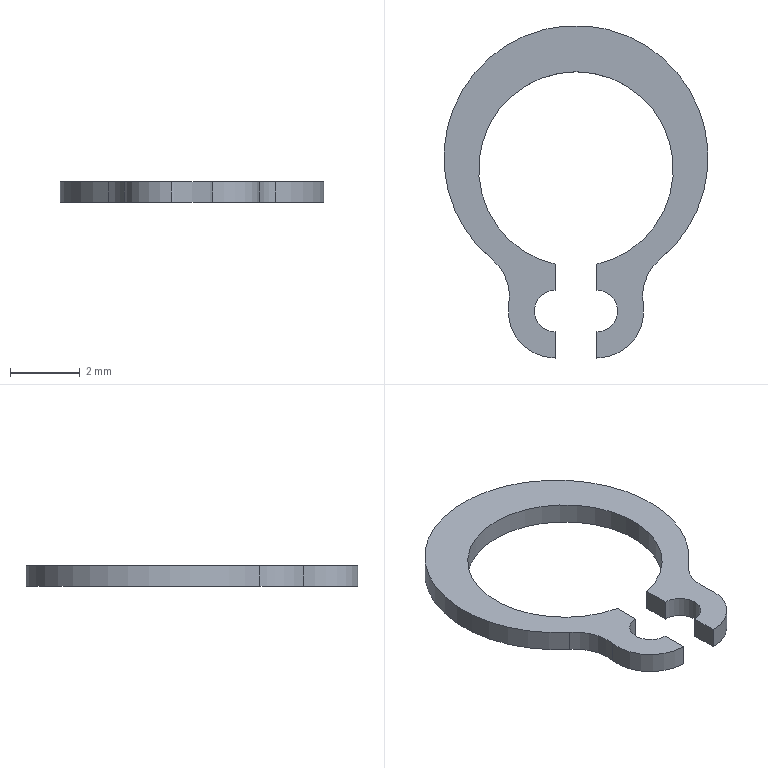Part | NX | features BREP 1, DATUM_CSYS 1 | 1 solid | 14 faces | box 7.6 x 9.565 x 0.6 mm | volume 14.427 mm3 | cylinder 8 | plane 6 | commonest cylinder face diameters 2.7 x4 1.2 x2 5.6 x1 7.6 x1
STEP:
#1=CARTESIAN_POINT('',(-0.6,-2.735,0.));
#2=VERTEX_POINT('',#1);
#3=CARTESIAN_POINT('',(0.6,-2.735,0.));
#4=VERTEX_POINT('',#3);
#5=CARTESIAN_POINT('',(0.,0.,0.));
#6=DIRECTION('',(0.,0.,-1.));
#7=DIRECTION('',(-0.2143,-0.9768,0.));
#8=AXIS2_PLACEMENT_3D('',#5,#6,#7);
#9=CIRCLE('',#8,2.8);
#10=EDGE_CURVE('',#2,#4,#9,.T.);
#11=ORIENTED_EDGE('',*,*,#10,.F.);
#12=CARTESIAN_POINT('',(-0.6,-3.485,0.));
#13=VERTEX_POINT('',#12);
#14=CARTESIAN_POINT('',(-0.6,-3.485,0.));
#15=DIRECTION('',(0.,1.,0.));
#16=VECTOR('',#15,1000.);
#17=LINE('',#14,#16);
#18=EDGE_CURVE('',#13,#2,#17,.T.);
#19=ORIENTED_EDGE('',*,*,#18,.F.);
#20=CARTESIAN_POINT('',(-0.6,-4.685,0.));
#21=VERTEX_POINT('',#20);
#22=CARTESIAN_POINT('',(-0.6,-4.085,0.));
#23=DIRECTION('',(0.,0.,-1.));
#24=DIRECTION('',(0.,-1.,0.));
#25=AXIS2_PLACEMENT_3D('',#22,#23,#24);
#26=CIRCLE('',#25,0.6);
#27=EDGE_CURVE('',#21,#13,#26,.T.);
#28=ORIENTED_EDGE('',*,*,#27,.F.);
#29=CARTESIAN_POINT('',(-0.6,-5.435,0.));
#30=VERTEX_POINT('',#29);
#31=CARTESIAN_POINT('',(-0.6,-5.435,0.));
#32=DIRECTION('',(0.,1.,0.));
#33=VECTOR('',#32,1000.);
#34=LINE('',#31,#33);
#35=EDGE_CURVE('',#30,#21,#34,.T.);
#36=ORIENTED_EDGE('',*,*,#35,.F.);
#37=CARTESIAN_POINT('',(-1.933,-3.869,0.));
#38=VERTEX_POINT('',#37);
#39=CARTESIAN_POINT('',(-0.6,-4.085,0.));
#40=DIRECTION('',(0.,0.,1.));
#41=DIRECTION('',(-0.9871,0.1601,0.));
#42=AXIS2_PLACEMENT_3D('',#39,#40,#41);
#43=CIRCLE('',#42,1.35);
#44=EDGE_CURVE('',#38,#30,#43,.T.);
#45=ORIENTED_EDGE('',*,*,#44,.F.);
#46=CARTESIAN_POINT('',(-2.409,-2.609,0.));
#47=VERTEX_POINT('',#46);
#48=CARTESIAN_POINT('',(-3.265,-3.653,0.));
#49=DIRECTION('',(0.,0.,-1.));
#50=DIRECTION('',(0.634,0.7733,0.));
#51=AXIS2_PLACEMENT_3D('',#48,#49,#50);
#52=CIRCLE('',#51,1.35);
#53=EDGE_CURVE('',#47,#38,#52,.T.);
#54=ORIENTED_EDGE('',*,*,#53,.F.);
#55=CARTESIAN_POINT('',(2.409,-2.609,0.));
#56=VERTEX_POINT('',#55);
#57=CARTESIAN_POINT('',(0.,0.33,0.));
#58=DIRECTION('',(0.,0.,1.));
#59=DIRECTION('',(0.634,-0.7733,0.));
#60=AXIS2_PLACEMENT_3D('',#57,#58,#59);
#61=CIRCLE('',#60,3.8);
#62=EDGE_CURVE('',#56,#47,#61,.T.);
#63=ORIENTED_EDGE('',*,*,#62,.F.);
#64=CARTESIAN_POINT('',(1.933,-3.869,0.));
#65=VERTEX_POINT('',#64);
#66=CARTESIAN_POINT('',(3.265,-3.653,0.));
#67=DIRECTION('',(0.,0.,-1.));
#68=DIRECTION('',(-0.9871,-0.1601,0.));
#69=AXIS2_PLACEMENT_3D('',#66,#67,#68);
#70=CIRCLE('',#69,1.35);
#71=EDGE_CURVE('',#65,#56,#70,.T.);
#72=ORIENTED_EDGE('',*,*,#71,.F.);
#73=CARTESIAN_POINT('',(0.6,-5.435,0.));
#74=VERTEX_POINT('',#73);
#75=CARTESIAN_POINT('',(0.6,-4.085,0.));
#76=DIRECTION('',(0.,0.,1.));
#77=DIRECTION('',(0.,-1.,0.));
#78=AXIS2_PLACEMENT_3D('',#75,#76,#77);
#79=CIRCLE('',#78,1.35);
#80=EDGE_CURVE('',#74,#65,#79,.T.);
#81=ORIENTED_EDGE('',*,*,#80,.F.);
#82=CARTESIAN_POINT('',(0.6,-4.685,0.));
#83=VERTEX_POINT('',#82);
#84=CARTESIAN_POINT('',(0.6,-4.685,0.));
#85=DIRECTION('',(0.,-1.,0.));
#86=VECTOR('',#85,1000.);
#87=LINE('',#84,#86);
#88=EDGE_CURVE('',#83,#74,#87,.T.);
#89=ORIENTED_EDGE('',*,*,#88,.F.);
#90=CARTESIAN_POINT('',(0.6,-3.485,0.));
#91=VERTEX_POINT('',#90);
#92=CARTESIAN_POINT('',(0.6,-4.085,0.));
#93=DIRECTION('',(0.,0.,-1.));
#94=DIRECTION('',(0.,1.,0.));
#95=AXIS2_PLACEMENT_3D('',#92,#93,#94);
#96=CIRCLE('',#95,0.6);
#97=EDGE_CURVE('',#91,#83,#96,.T.);
#98=ORIENTED_EDGE('',*,*,#97,.F.);
#99=CARTESIAN_POINT('',(0.6,-2.735,0.));
#100=DIRECTION('',(0.,-1.,0.));
#101=VECTOR('',#100,1000.);
#102=LINE('',#99,#101);
#103=EDGE_CURVE('',#4,#91,#102,.T.);
#104=ORIENTED_EDGE('',*,*,#103,.F.);
#105=EDGE_LOOP('',(#11,#19,#28,#36,#45,#54,#63,#72,#81,#89,#98,#104));
#106=FACE_BOUND('',#105,.T.);
#107=CARTESIAN_POINT('',(0.3031,-0.6525,0.));
#108=DIRECTION('',(0.,0.,1.));
#109=DIRECTION('',(-1.,0.,0.));
#110=AXIS2_PLACEMENT_3D('',#107,#108,#109);
#111=PLANE('',#110);
#112=ADVANCED_FACE('',(#106),#111,.F.);
#113=CARTESIAN_POINT('',(0.6,-2.735,0.6));
#114=VERTEX_POINT('',#113);
#115=CARTESIAN_POINT('',(0.6,-3.485,0.6));
#116=VERTEX_POINT('',#115);
#117=CARTESIAN_POINT('',(0.6,-2.735,0.6));
#118=DIRECTION('',(0.,-1.,0.));
#119=VECTOR('',#118,1000.);
#120=LINE('',#117,#119);
#121=EDGE_CURVE('',#114,#116,#120,.T.);
#122=ORIENTED_EDGE('',*,*,#121,.T.);
#123=CARTESIAN_POINT('',(0.6,-4.685,0.6));
#124=VERTEX_POINT('',#123);
#125=CARTESIAN_POINT('',(0.6,-4.085,0.6));
#126=DIRECTION('',(0.,0.,-1.));
#127=DIRECTION('',(0.,1.,0.));
#128=AXIS2_PLACEMENT_3D('',#125,#126,#127);
#129=CIRCLE('',#128,0.6);
#130=EDGE_CURVE('',#116,#124,#129,.T.);
#131=ORIENTED_EDGE('',*,*,#130,.T.);
#132=CARTESIAN_POINT('',(0.6,-5.435,0.6));
#133=VERTEX_POINT('',#132);
#134=CARTESIAN_POINT('',(0.6,-4.685,0.6));
#135=DIRECTION('',(0.,-1.,0.));
#136=VECTOR('',#135,1000.);
#137=LINE('',#134,#136);
#138=EDGE_CURVE('',#124,#133,#137,.T.);
#139=ORIENTED_EDGE('',*,*,#138,.T.);
#140=CARTESIAN_POINT('',(1.933,-3.869,0.6));
#141=VERTEX_POINT('',#140);
#142=CARTESIAN_POINT('',(0.6,-4.085,0.6));
#143=DIRECTION('',(0.,0.,1.));
#144=DIRECTION('',(0.,-1.,0.));
#145=AXIS2_PLACEMENT_3D('',#142,#143,#144);
#146=CIRCLE('',#145,1.35);
#147=EDGE_CURVE('',#133,#141,#146,.T.);
#148=ORIENTED_EDGE('',*,*,#147,.T.);
#149=CARTESIAN_POINT('',(2.409,-2.609,0.6));
#150=VERTEX_POINT('',#149);
#151=CARTESIAN_POINT('',(3.265,-3.653,0.6));
#152=DIRECTION('',(0.,0.,-1.));
#153=DIRECTION('',(-0.9871,-0.1601,0.));
#154=AXIS2_PLACEMENT_3D('',#151,#152,#153);
#155=CIRCLE('',#154,1.35);
#156=EDGE_CURVE('',#141,#150,#155,.T.);
#157=ORIENTED_EDGE('',*,*,#156,.T.);
#158=CARTESIAN_POINT('',(-2.409,-2.609,0.6));
#159=VERTEX_POINT('',#158);
#160=CARTESIAN_POINT('',(0.,0.33,0.6));
#161=DIRECTION('',(0.,0.,1.));
#162=DIRECTION('',(0.634,-0.7733,0.));
#163=AXIS2_PLACEMENT_3D('',#160,#161,#162);
#164=CIRCLE('',#163,3.8);
#165=EDGE_CURVE('',#150,#159,#164,.T.);
#166=ORIENTED_EDGE('',*,*,#165,.T.);
#167=CARTESIAN_POINT('',(-1.933,-3.869,0.6));
#168=VERTEX_POINT('',#167);
#169=CARTESIAN_POINT('',(-3.265,-3.653,0.6));
#170=DIRECTION('',(0.,0.,-1.));
#171=DIRECTION('',(0.634,0.7733,0.));
#172=AXIS2_PLACEMENT_3D('',#169,#170,#171);
#173=CIRCLE('',#172,1.35);
#174=EDGE_CURVE('',#159,#168,#173,.T.);
#175=ORIENTED_EDGE('',*,*,#174,.T.);
#176=CARTESIAN_POINT('',(-0.6,-5.435,0.6));
#177=VERTEX_POINT('',#176);
#178=CARTESIAN_POINT('',(-0.6,-4.085,0.6));
#179=DIRECTION('',(0.,0.,1.));
#180=DIRECTION('',(-0.9871,0.1601,0.));
#181=AXIS2_PLACEMENT_3D('',#178,#179,#180);
#182=CIRCLE('',#181,1.35);
#183=EDGE_CURVE('',#168,#177,#182,.T.);
#184=ORIENTED_EDGE('',*,*,#183,.T.);
#185=CARTESIAN_POINT('',(-0.6,-4.685,0.6));
#186=VERTEX_POINT('',#185);
#187=CARTESIAN_POINT('',(-0.6,-5.435,0.6));
#188=DIRECTION('',(0.,1.,0.));
#189=VECTOR('',#188,1000.);
#190=LINE('',#187,#189);
#191=EDGE_CURVE('',#177,#186,#190,.T.);
#192=ORIENTED_EDGE('',*,*,#191,.T.);
#193=CARTESIAN_POINT('',(-0.6,-3.485,0.6));
#194=VERTEX_POINT('',#193);
#195=CARTESIAN_POINT('',(-0.6,-4.085,0.6));
#196=DIRECTION('',(0.,0.,-1.));
#197=DIRECTION('',(0.,-1.,0.));
#198=AXIS2_PLACEMENT_3D('',#195,#196,#197);
#199=CIRCLE('',#198,0.6);
#200=EDGE_CURVE('',#186,#194,#199,.T.);
#201=ORIENTED_EDGE('',*,*,#200,.T.);
#202=CARTESIAN_POINT('',(-0.6,-2.735,0.6));
#203=VERTEX_POINT('',#202);
#204=CARTESIAN_POINT('',(-0.6,-3.485,0.6));
#205=DIRECTION('',(0.,1.,0.));
#206=VECTOR('',#205,1000.);
#207=LINE('',#204,#206);
#208=EDGE_CURVE('',#194,#203,#207,.T.);
#209=ORIENTED_EDGE('',*,*,#208,.T.);
#210=CARTESIAN_POINT('',(0.,0.,0.6));
#211=DIRECTION('',(0.,0.,-1.));
#212=DIRECTION('',(-0.2143,-0.9768,0.));
#213=AXIS2_PLACEMENT_3D('',#210,#211,#212);
#214=CIRCLE('',#213,2.8);
#215=EDGE_CURVE('',#203,#114,#214,.T.);
#216=ORIENTED_EDGE('',*,*,#215,.T.);
#217=EDGE_LOOP('',(#122,#131,#139,#148,#157,#166,#175,#184,#192,#201,#209,#216));
#218=FACE_BOUND('',#217,.T.);
#219=CARTESIAN_POINT('',(0.3031,-0.6525,0.6));
#220=DIRECTION('',(0.,0.,1.));
#221=DIRECTION('',(-1.,0.,0.));
#222=AXIS2_PLACEMENT_3D('',#219,#220,#221);
#223=PLANE('',#222);
#224=ADVANCED_FACE('',(#218),#223,.T.);
#225=ORIENTED_EDGE('',*,*,#103,.T.);
#226=CARTESIAN_POINT('',(0.6,-3.485,0.));
#227=DIRECTION('',(0.,0.,1.));
#228=VECTOR('',#227,1000.);
#229=LINE('',#226,#228);
#230=EDGE_CURVE('',#91,#116,#229,.T.);
#231=ORIENTED_EDGE('',*,*,#230,.T.);
#232=ORIENTED_EDGE('',*,*,#121,.F.);
#233=CARTESIAN_POINT('',(0.6,-2.735,0.));
#234=DIRECTION('',(0.,0.,1.));
#235=VECTOR('',#234,1000.);
#236=LINE('',#233,#235);
#237=EDGE_CURVE('',#4,#114,#236,.T.);
#238=ORIENTED_EDGE('',*,*,#237,.F.);
#239=EDGE_LOOP('',(#225,#231,#232,#238));
#240=FACE_BOUND('',#239,.T.);
#241=CARTESIAN_POINT('',(0.6,-3.11,0.3));
#242=DIRECTION('',(-1.,0.,0.));
#243=DIRECTION('',(0.,1.,0.));
#244=AXIS2_PLACEMENT_3D('',#241,#242,#243);
#245=PLANE('',#244);
#246=ADVANCED_FACE('',(#240),#245,.T.);
#247=ORIENTED_EDGE('',*,*,#97,.T.);
#248=CARTESIAN_POINT('',(0.6,-4.685,0.));
#249=DIRECTION('',(0.,0.,1.));
#250=VECTOR('',#249,1000.);
#251=LINE('',#248,#250);
#252=EDGE_CURVE('',#83,#124,#251,.T.);
#253=ORIENTED_EDGE('',*,*,#252,.T.);
#254=ORIENTED_EDGE('',*,*,#130,.F.);
#255=ORIENTED_EDGE('',*,*,#230,.F.);
#256=EDGE_LOOP('',(#247,#253,#254,#255));
#257=FACE_BOUND('',#256,.T.);
#258=CARTESIAN_POINT('',(0.6,-4.085,0.));
#259=DIRECTION('',(0.,0.,1.));
#260=DIRECTION('',(0.,-1.,0.));
#261=AXIS2_PLACEMENT_3D('',#258,#259,#260);
#262=CYLINDRICAL_SURFACE('',#261,0.6);
#263=ADVANCED_FACE('',(#257),#262,.F.);
#264=ORIENTED_EDGE('',*,*,#88,.T.);
#265=CARTESIAN_POINT('',(0.6,-5.435,0.));
#266=DIRECTION('',(0.,0.,1.));
#267=VECTOR('',#266,1000.);
#268=LINE('',#265,#267);
#269=EDGE_CURVE('',#74,#133,#268,.T.);
#270=ORIENTED_EDGE('',*,*,#269,.T.);
#271=ORIENTED_EDGE('',*,*,#138,.F.);
#272=ORIENTED_EDGE('',*,*,#252,.F.);
#273=EDGE_LOOP('',(#264,#270,#271,#272));
#274=FACE_BOUND('',#273,.T.);
#275=CARTESIAN_POINT('',(0.6,-5.06,0.3));
#276=DIRECTION('',(-1.,0.,0.));
#277=DIRECTION('',(0.,1.,0.));
#278=AXIS2_PLACEMENT_3D('',#275,#276,#277);
#279=PLANE('',#278);
#280=ADVANCED_FACE('',(#274),#279,.T.);
#281=ORIENTED_EDGE('',*,*,#80,.T.);
#282=CARTESIAN_POINT('',(1.933,-3.869,0.));
#283=DIRECTION('',(0.,0.,1.));
#284=VECTOR('',#283,1000.);
#285=LINE('',#282,#284);
#286=EDGE_CURVE('',#65,#141,#285,.T.);
#287=ORIENTED_EDGE('',*,*,#286,.T.);
#288=ORIENTED_EDGE('',*,*,#147,.F.);
#289=ORIENTED_EDGE('',*,*,#269,.F.);
#290=EDGE_LOOP('',(#281,#287,#288,#289));
#291=FACE_BOUND('',#290,.T.);
#292=CARTESIAN_POINT('',(0.6,-4.085,0.));
#293=DIRECTION('',(0.,0.,1.));
#294=DIRECTION('',(0.,1.,0.));
#295=AXIS2_PLACEMENT_3D('',#292,#293,#294);
#296=CYLINDRICAL_SURFACE('',#295,1.35);
#297=ADVANCED_FACE('',(#291),#296,.T.);
#298=ORIENTED_EDGE('',*,*,#71,.T.);
#299=CARTESIAN_POINT('',(2.409,-2.609,0.));
#300=DIRECTION('',(0.,0.,1.));
#301=VECTOR('',#300,1000.);
#302=LINE('',#299,#301);
#303=EDGE_CURVE('',#56,#150,#302,.T.);
#304=ORIENTED_EDGE('',*,*,#303,.T.);
#305=ORIENTED_EDGE('',*,*,#156,.F.);
#306=ORIENTED_EDGE('',*,*,#286,.F.);
#307=EDGE_LOOP('',(#298,#304,#305,#306));
#308=FACE_BOUND('',#307,.T.);
#309=CARTESIAN_POINT('',(3.265,-3.653,0.));
#310=DIRECTION('',(0.,0.,1.));
#311=DIRECTION('',(0.9871,0.1601,0.));
#312=AXIS2_PLACEMENT_3D('',#309,#310,#311);
#313=CYLINDRICAL_SURFACE('',#312,1.35);
#314=ADVANCED_FACE('',(#308),#313,.F.);
#315=ORIENTED_EDGE('',*,*,#303,.F.);
#316=ORIENTED_EDGE('',*,*,#62,.T.);
#317=CARTESIAN_POINT('',(-2.409,-2.609,0.));
#318=DIRECTION('',(0.,0.,1.));
#319=VECTOR('',#318,1000.);
#320=LINE('',#317,#319);
#321=EDGE_CURVE('',#47,#159,#320,.T.);
#322=ORIENTED_EDGE('',*,*,#321,.T.);
#323=ORIENTED_EDGE('',*,*,#165,.F.);
#324=EDGE_LOOP('',(#315,#316,#322,#323));
#325=FACE_BOUND('',#324,.T.);
#326=CARTESIAN_POINT('',(0.,0.33,0.));
#327=DIRECTION('',(0.,0.,1.));
#328=DIRECTION('',(-0.634,0.7733,0.));
#329=AXIS2_PLACEMENT_3D('',#326,#327,#328);
#330=CYLINDRICAL_SURFACE('',#329,3.8);
#331=ADVANCED_FACE('',(#325),#330,.T.);
#332=ORIENTED_EDGE('',*,*,#53,.T.);
#333=CARTESIAN_POINT('',(-1.933,-3.869,0.));
#334=DIRECTION('',(0.,0.,1.));
#335=VECTOR('',#334,1000.);
#336=LINE('',#333,#335);
#337=EDGE_CURVE('',#38,#168,#336,.T.);
#338=ORIENTED_EDGE('',*,*,#337,.T.);
#339=ORIENTED_EDGE('',*,*,#174,.F.);
#340=ORIENTED_EDGE('',*,*,#321,.F.);
#341=EDGE_LOOP('',(#332,#338,#339,#340));
#342=FACE_BOUND('',#341,.T.);
#343=CARTESIAN_POINT('',(-3.265,-3.653,0.));
#344=DIRECTION('',(0.,0.,1.));
#345=DIRECTION('',(-0.634,-0.7733,0.));
#346=AXIS2_PLACEMENT_3D('',#343,#344,#345);
#347=CYLINDRICAL_SURFACE('',#346,1.35);
#348=ADVANCED_FACE('',(#342),#347,.F.);
#349=ORIENTED_EDGE('',*,*,#44,.T.);
#350=CARTESIAN_POINT('',(-0.6,-5.435,0.));
#351=DIRECTION('',(0.,0.,1.));
#352=VECTOR('',#351,1000.);
#353=LINE('',#350,#352);
#354=EDGE_CURVE('',#30,#177,#353,.T.);
#355=ORIENTED_EDGE('',*,*,#354,.T.);
#356=ORIENTED_EDGE('',*,*,#183,.F.);
#357=ORIENTED_EDGE('',*,*,#337,.F.);
#358=EDGE_LOOP('',(#349,#355,#356,#357));
#359=FACE_BOUND('',#358,.T.);
#360=CARTESIAN_POINT('',(-0.6,-4.085,0.));
#361=DIRECTION('',(0.,0.,1.));
#362=DIRECTION('',(0.9871,-0.1601,0.));
#363=AXIS2_PLACEMENT_3D('',#360,#361,#362);
#364=CYLINDRICAL_SURFACE('',#363,1.35);
#365=ADVANCED_FACE('',(#359),#364,.T.);
#366=ORIENTED_EDGE('',*,*,#35,.T.);
#367=CARTESIAN_POINT('',(-0.6,-4.685,0.));
#368=DIRECTION('',(0.,0.,1.));
#369=VECTOR('',#368,1000.);
#370=LINE('',#367,#369);
#371=EDGE_CURVE('',#21,#186,#370,.T.);
#372=ORIENTED_EDGE('',*,*,#371,.T.);
#373=ORIENTED_EDGE('',*,*,#191,.F.);
#374=ORIENTED_EDGE('',*,*,#354,.F.);
#375=EDGE_LOOP('',(#366,#372,#373,#374));
#376=FACE_BOUND('',#375,.T.);
#377=CARTESIAN_POINT('',(-0.6,-5.06,0.3));
#378=DIRECTION('',(1.,0.,0.));
#379=DIRECTION('',(0.,-1.,0.));
#380=AXIS2_PLACEMENT_3D('',#377,#378,#379);
#381=PLANE('',#380);
#382=ADVANCED_FACE('',(#376),#381,.T.);
#383=ORIENTED_EDGE('',*,*,#27,.T.);
#384=CARTESIAN_POINT('',(-0.6,-3.485,0.));
#385=DIRECTION('',(0.,0.,1.));
#386=VECTOR('',#385,1000.);
#387=LINE('',#384,#386);
#388=EDGE_CURVE('',#13,#194,#387,.T.);
#389=ORIENTED_EDGE('',*,*,#388,.T.);
#390=ORIENTED_EDGE('',*,*,#200,.F.);
#391=ORIENTED_EDGE('',*,*,#371,.F.);
#392=EDGE_LOOP('',(#383,#389,#390,#391));
#393=FACE_BOUND('',#392,.T.);
#394=CARTESIAN_POINT('',(-0.6,-4.085,0.));
#395=DIRECTION('',(0.,0.,1.));
#396=DIRECTION('',(0.,1.,0.));
#397=AXIS2_PLACEMENT_3D('',#394,#395,#396);
#398=CYLINDRICAL_SURFACE('',#397,0.6);
#399=ADVANCED_FACE('',(#393),#398,.F.);
#400=ORIENTED_EDGE('',*,*,#18,.T.);
#401=CARTESIAN_POINT('',(-0.6,-2.735,0.));
#402=DIRECTION('',(0.,0.,1.));
#403=VECTOR('',#402,1000.);
#404=LINE('',#401,#403);
#405=EDGE_CURVE('',#2,#203,#404,.T.);
#406=ORIENTED_EDGE('',*,*,#405,.T.);
#407=ORIENTED_EDGE('',*,*,#208,.F.);
#408=ORIENTED_EDGE('',*,*,#388,.F.);
#409=EDGE_LOOP('',(#400,#406,#407,#408));
#410=FACE_BOUND('',#409,.T.);
#411=CARTESIAN_POINT('',(-0.6,-3.11,0.3));
#412=DIRECTION('',(1.,0.,0.));
#413=DIRECTION('',(0.,-1.,0.));
#414=AXIS2_PLACEMENT_3D('',#411,#412,#413);
#415=PLANE('',#414);
#416=ADVANCED_FACE('',(#410),#415,.T.);
#417=ORIENTED_EDGE('',*,*,#10,.T.);
#418=ORIENTED_EDGE('',*,*,#237,.T.);
#419=ORIENTED_EDGE('',*,*,#215,.F.);
#420=ORIENTED_EDGE('',*,*,#405,.F.);
#421=EDGE_LOOP('',(#417,#418,#419,#420));
#422=FACE_BOUND('',#421,.T.);
#423=CARTESIAN_POINT('',(0.,0.,0.));
#424=DIRECTION('',(0.,0.,1.));
#425=DIRECTION('',(-0.2143,0.9768,0.));
#426=AXIS2_PLACEMENT_3D('',#423,#424,#425);
#427=CYLINDRICAL_SURFACE('',#426,2.8);
#428=ADVANCED_FACE('',(#422),#427,.F.);
#429=CLOSED_SHELL('',(#112,#224,#246,#263,#280,#297,#314,#331,#348,#365,#382,#399,#416,#428));
#430=MANIFOLD_SOLID_BREP('',#429);
#431=(LENGTH_UNIT()NAMED_UNIT(*)SI_UNIT(.MILLI.,.METRE.));
#432=UNCERTAINTY_MEASURE_WITH_UNIT(LENGTH_MEASURE(0.00001),#431,'','');
#433=(NAMED_UNIT(*)PLANE_ANGLE_UNIT()SI_UNIT($,.RADIAN.));
#434=(NAMED_UNIT(*)SI_UNIT($,.STERADIAN.)SOLID_ANGLE_UNIT());
#435=(GEOMETRIC_REPRESENTATION_CONTEXT(3)GLOBAL_UNCERTAINTY_ASSIGNED_CONTEXT((#432))GLOBAL_UNIT_ASSIGNED_CONTEXT((#431,#433,#434))REPRESENTATION_CONTEXT('',''));
#436=ADVANCED_BREP_SHAPE_REPRESENTATION('',(#430),#435);